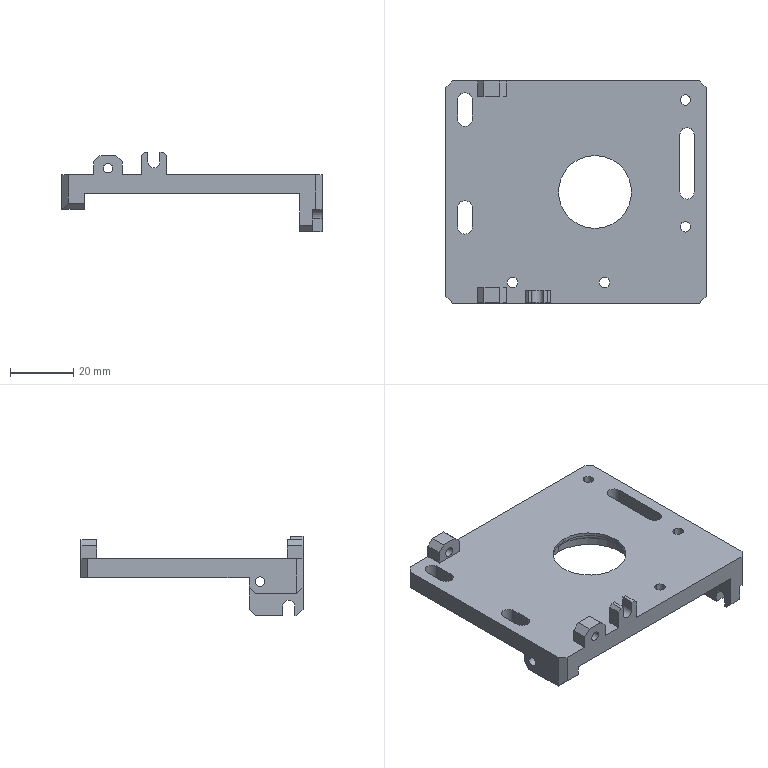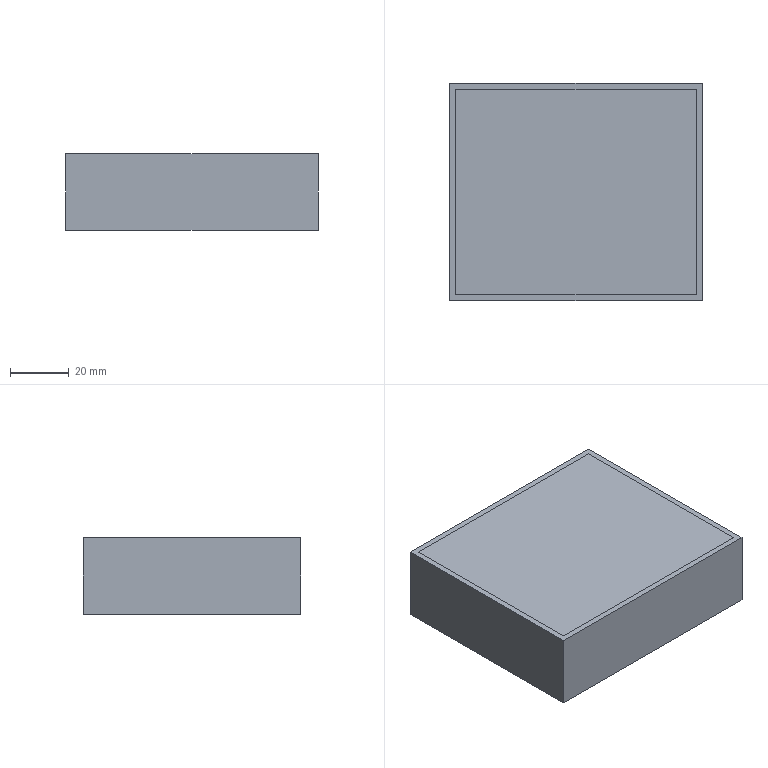CAM job | NX | 3-axis milling, drilling | part box 82 x 70 x 25 mm | stock box 86 x 74 x 26 mm
Tools:
number,name,description,diameter,corner_radius,flute_length,length,flutes
1,D20R0.8,Milling Tool-5 Parameters,20.0,0.8,50.0,75.0,2
6,D6,Milling Tool-5 Parameters,6.0,0.0,50.0,75.0,2
10,D10,Milling Tool-5 Parameters,10.0,0.0,50.0,75.0,2
4,D4,Milling Tool-5 Parameters,4.0,0.0,50.0,75.0,2
3,D3,Milling Tool-5 Parameters,3.0,0.0,50.0,75.0,2
2,R1,Milling Tool-5 Parameters,2.0,1.0,50.0,75.0,2
7,D6A45,Milling Tool-5 Parameters,6.0,0.0,50.0,75.0,2
9,3.3ZT,Drilling Tool,3.3,0.0,35.0,50.0,2
8,D2,Milling Tool-5 Parameters,2.0,0.0,50.0,75.0,2
12,T6H1,Milling Tool-T Cutter,6.0,,1.0,25.0,4
13,D2.4XYD,Thread Mill,2.4,0.0,0.5,50.0,2
Operations:
program,operation,operation_type,tool,method,geometry_group,spindle_rpm,surface_speed,feed_per_tooth,feed_cut,feed_plunge,cut_length_mm,path_length_mm,cut_time_min,machine_time_min
1,FLOOR_WALL,VolumeBased25DMillingOperation,D20R0.8,METHOD,A,7500.0,471.0,0.09,1350.0,100.0,926.639,980.639,0.6864,0.6918
1,ZLEVEL_PROFILE_1,ZLevelMilling,D6,METHOD,A,9500.0,179.0,0.1579,3000.0,1000.0,26831.561,26913.511,8.967,8.975
1,ZLEVEL_PROFILE_COPY,ZLevelMilling,D6,METHOD,A,9500.0,179.0,0.0789,1500.0,1000.0,1197.103,1287.37,0.7987,0.8077
1,CAVITY_MILL,CavityMilling,D10,METHOD,A,9500.0,298.0,0.1579,3000.0,100.0,36967.915,37304.502,12.323,12.356
1,CAVITY_MILL_COPY,CavityMilling,D4,METHOD,A,9500.0,119.0,0.0947,1800.0,100.0,1029.974,1541.456,0.5722,0.6234
1,FLOOR_WALL_1,VolumeBased25DMillingOperation,D4,METHOD,A,9500.0,119.0,0.0711,1350.0,100.0,3311.302,4347.785,2.453,2.557
1,CAVITY_MILL_COPY_COPY,CavityMilling,D3,METHOD,A,9500.0,119.0,0.0947,1800.0,100.0,323.692,557.121,0.1798,0.2032
1,FIXED_CONTOUR,SurfaceContour,R1,METHOD,A,9500.0,59.0,0.1474,2800.0,100.0,1139.004,1582.621,0.4068,0.4511
1,PLANAR_MILL_COPY,PlanarMilling,D6A45,METHOD,A,9500.0,179.0,0.0658,1250.0,500.0,278.128,435.311,0.2337,0.2495
2,FLOOR_WALL_COPY,VolumeBased25DMillingOperation,D20R0.8,METHOD,B,7500.0,471.0,0.09,1350.0,100.0,890.639,944.639,0.6597,0.6651
2,CAVITY_MILL_COPY_1,CavityMilling,D10,METHOD,B,9500.0,298.0,0.1579,3000.0,100.0,29629.204,29926.942,9.876,9.906
2,CAVITY_MILL_COPY_1_COPY,CavityMilling,D10,METHOD,B,9500.0,298.0,0.1579,3000.0,100.0,1380.14,1764.159,0.46,0.4984
2,FLOOR_WALL_1_COPY,VolumeBased25DMillingOperation,D4,METHOD,B,9500.0,119.0,0.0711,1350.0,100.0,3222.858,3682.319,2.387,2.433
2,FLOOR_WALL_1_COPY_COPY_1,VolumeBased25DMillingOperation,D4,METHOD,B,9500.0,119.0,0.0711,1350.0,100.0,145.801,330.051,0.108,0.1264
2,ZLEVEL_PROFILE_COPY_COPY,ZLevelMilling,D4,METHOD,B,9500.0,179.0,0.0789,1500.0,1000.0,227.355,317.855,0.1522,0.1612
2,ZLEVEL_PROFILE_1_1,ZLevelMilling,D3,METHOD,B,9500.0,89.0,0.0684,1300.0,1000.0,2347.253,2714.803,1.821,1.858
2,CAVITY_MILL_COPY_COPY_COPY,CavityMilling,D3,METHOD,B,9500.0,119.0,0.0789,1500.0,100.0,667.29,985.14,0.4449,0.4766
2,FLOOR_WALL_1_COPY_COPY,VolumeBased25DMillingOperation,D2,METHOD,B,9500.0,59.0,0.0711,1350.0,100.0,609.224,986.811,0.4513,0.489
2,FIXED_CONTOUR_COPY,SurfaceContour,R1,METHOD,B,9500.0,59.0,0.1474,2800.0,100.0,1899.554,2318.112,0.6784,0.7203
2,DRILLING,Operation,D6A45,METHOD,B,5000.0,94.0,0.025,250.0,0.0,20.1,233.54,0.0804,0.1017
2,DRILLING_COPY_COPY,Operation,3.3ZT,METHOD,B,2000.0,20.0,0.0375,150.0,0.0,45.966,285.271,0.3064,0.3304
2,PLANAR_MILL,PlanarMilling,D6A45,METHOD,B,9500.0,179.0,0.0658,1250.0,500.0,396.894,942.113,0.3465,0.4011
2,PLANAR_MILL_COPY_1,PlanarMilling,D6A45,METHOD,B,9500.0,179.0,0.0658,1250.0,500.0,75.826,155.827,0.0746,0.0826
2,PLANAR_MILL_1,PlanarMilling,T6H1,METHOD,B,7000.0,131.0,0.0446,1250.0,100.0,293.335,382.335,0.2347,0.2436
2,THREAD_MILLING,ThreadMilling,D2.4XYD,METHOD,B,5000.0,157.0,0.125,1250.0,100.0,1517.359,1609.389,1.214,1.223